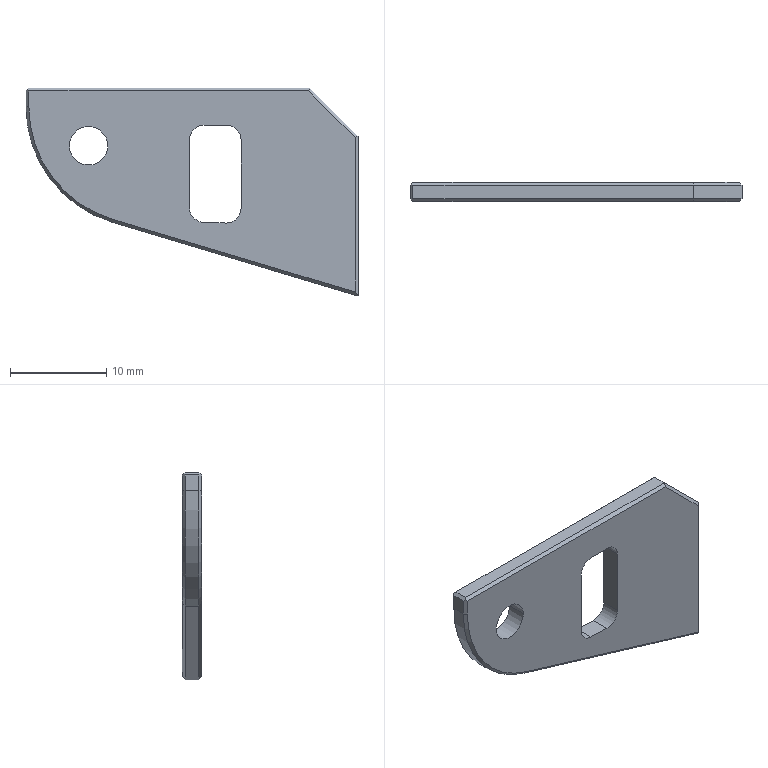Part | NX | 1 solid | 31 faces | box 34.5 x 2 x 21.6 mm | volume 937.237 mm3 | plane 22 | cylinder 7 | cone 2 | commonest cylinder face diameters 3 x4 4 x2 25 x1
STEP:
#1=CARTESIAN_POINT('',(-158.,156.8,-48.85));
#2=VERTEX_POINT('',#1);
#3=CARTESIAN_POINT('',(-158.,156.8,-47.2));
#4=VERTEX_POINT('',#3);
#5=CARTESIAN_POINT('',(-158.,156.8,-48.025));
#6=DIRECTION('',(0.,0.,1.));
#7=VECTOR('',#6,1000.);
#8=LINE('',#5,#7);
#9=EDGE_CURVE('',#2,#4,#8,.T.);
#10=ORIENTED_EDGE('',*,*,#9,.T.);
#11=CARTESIAN_POINT('',(-158.,158.2,-47.2));
#12=VERTEX_POINT('',#11);
#13=CARTESIAN_POINT('',(-158.,157.35,-47.2));
#14=DIRECTION('',(0.,1.,0.));
#15=VECTOR('',#14,1000.);
#16=LINE('',#13,#15);
#17=EDGE_CURVE('',#4,#12,#16,.T.);
#18=ORIENTED_EDGE('',*,*,#17,.T.);
#19=CARTESIAN_POINT('',(-158.,158.2,-48.85));
#20=VERTEX_POINT('',#19);
#21=CARTESIAN_POINT('',(-158.,158.2,-48.025));
#22=DIRECTION('',(0.,0.,1.));
#23=VECTOR('',#22,1000.);
#24=LINE('',#21,#23);
#25=EDGE_CURVE('',#20,#12,#24,.T.);
#26=ORIENTED_EDGE('',*,*,#25,.F.);
#27=CARTESIAN_POINT('',(-158.,156.5,-48.85));
#28=DIRECTION('',(0.,1.,0.));
#29=VECTOR('',#28,1000.);
#30=LINE('',#27,#29);
#31=EDGE_CURVE('',#2,#20,#30,.T.);
#32=ORIENTED_EDGE('',*,*,#31,.F.);
#33=EDGE_LOOP('',(#10,#18,#26,#32));
#34=FACE_BOUND('',#33,.T.);
#35=CARTESIAN_POINT('',(-158.,156.5,-42.9));
#36=DIRECTION('',(-1.,0.,0.));
#37=DIRECTION('',(0.,0.,1.));
#38=AXIS2_PLACEMENT_3D('',#35,#36,#37);
#39=PLANE('',#38);
#40=ADVANCED_FACE('',(#34),#39,.T.);
#41=CARTESIAN_POINT('',(-157.7,156.8,-46.9));
#42=VERTEX_POINT('',#41);
#43=CARTESIAN_POINT('',(-128.5,156.8,-46.9));
#44=VERTEX_POINT('',#43);
#45=CARTESIAN_POINT('',(-143.462,156.8,-46.9));
#46=DIRECTION('',(1.,0.,0.));
#47=VECTOR('',#46,1000.);
#48=LINE('',#45,#47);
#49=EDGE_CURVE('',#42,#44,#48,.T.);
#50=ORIENTED_EDGE('',*,*,#49,.T.);
#51=CARTESIAN_POINT('',(-128.5,158.2,-46.9));
#52=VERTEX_POINT('',#51);
#53=CARTESIAN_POINT('',(-128.5,157.5,-46.9));
#54=DIRECTION('',(0.,1.,0.));
#55=VECTOR('',#54,1000.);
#56=LINE('',#53,#55);
#57=EDGE_CURVE('',#44,#52,#56,.T.);
#58=ORIENTED_EDGE('',*,*,#57,.T.);
#59=CARTESIAN_POINT('',(-157.7,158.2,-46.9));
#60=VERTEX_POINT('',#59);
#61=CARTESIAN_POINT('',(-108.092,158.2,-46.9));
#62=DIRECTION('',(1.,0.,0.));
#63=VECTOR('',#62,1000.);
#64=LINE('',#61,#63);
#65=EDGE_CURVE('',#60,#52,#64,.T.);
#66=ORIENTED_EDGE('',*,*,#65,.F.);
#67=CARTESIAN_POINT('',(-157.7,157.35,-46.9));
#68=DIRECTION('',(0.,1.,0.));
#69=VECTOR('',#68,1000.);
#70=LINE('',#67,#69);
#71=EDGE_CURVE('',#42,#60,#70,.T.);
#72=ORIENTED_EDGE('',*,*,#71,.F.);
#73=EDGE_LOOP('',(#50,#58,#66,#72));
#74=FACE_BOUND('',#73,.T.);
#75=CARTESIAN_POINT('',(-123.5,156.5,-46.9));
#76=DIRECTION('',(0.,0.,1.));
#77=DIRECTION('',(0.,-1.,0.));
#78=AXIS2_PLACEMENT_3D('',#75,#76,#77);
#79=PLANE('',#78);
#80=ADVANCED_FACE('',(#74),#79,.T.);
#81=CARTESIAN_POINT('',(-123.5,158.2,-68.5));
#82=VERTEX_POINT('',#81);
#83=CARTESIAN_POINT('',(-123.5,156.8,-68.5));
#84=VERTEX_POINT('',#83);
#85=CARTESIAN_POINT('',(-123.5,156.5,-68.5));
#86=DIRECTION('',(0.,-1.,0.));
#87=VECTOR('',#86,1000.);
#88=LINE('',#85,#87);
#89=EDGE_CURVE('',#82,#84,#88,.T.);
#90=ORIENTED_EDGE('',*,*,#89,.F.);
#91=CARTESIAN_POINT('',(-123.5,158.2,-51.9));
#92=VERTEX_POINT('',#91);
#93=CARTESIAN_POINT('',(-123.5,158.2,-60.412));
#94=DIRECTION('',(0.,0.,-1.));
#95=VECTOR('',#94,1000.);
#96=LINE('',#93,#95);
#97=EDGE_CURVE('',#92,#82,#96,.T.);
#98=ORIENTED_EDGE('',*,*,#97,.F.);
#99=CARTESIAN_POINT('',(-123.5,156.8,-51.9));
#100=VERTEX_POINT('',#99);
#101=CARTESIAN_POINT('',(-123.5,157.5,-51.9));
#102=DIRECTION('',(0.,1.,0.));
#103=VECTOR('',#102,1000.);
#104=LINE('',#101,#103);
#105=EDGE_CURVE('',#100,#92,#104,.T.);
#106=ORIENTED_EDGE('',*,*,#105,.F.);
#107=CARTESIAN_POINT('',(-123.5,156.8,-60.412));
#108=DIRECTION('',(0.,0.,-1.));
#109=VECTOR('',#108,1000.);
#110=LINE('',#107,#109);
#111=EDGE_CURVE('',#100,#84,#110,.T.);
#112=ORIENTED_EDGE('',*,*,#111,.T.);
#113=EDGE_LOOP('',(#90,#98,#106,#112));
#114=FACE_BOUND('',#113,.T.);
#115=CARTESIAN_POINT('',(-123.5,156.5,-67.9));
#116=DIRECTION('',(1.,0.,0.));
#117=DIRECTION('',(0.,1.,0.));
#118=AXIS2_PLACEMENT_3D('',#115,#116,#117);
#119=PLANE('',#118);
#120=ADVANCED_FACE('',(#114),#119,.T.);
#121=CARTESIAN_POINT('',(-135.65,156.5,-59.427));
#122=VERTEX_POINT('',#121);
#123=CARTESIAN_POINT('',(-135.65,158.5,-59.427));
#124=VERTEX_POINT('',#123);
#125=CARTESIAN_POINT('',(-135.65,156.5,-59.427));
#126=DIRECTION('',(0.,1.,0.));
#127=VECTOR('',#126,1000.);
#128=LINE('',#125,#127);
#129=EDGE_CURVE('',#122,#124,#128,.T.);
#130=ORIENTED_EDGE('',*,*,#129,.T.);
#131=CARTESIAN_POINT('',(-137.197,158.5,-60.926));
#132=VERTEX_POINT('',#131);
#133=CARTESIAN_POINT('',(-137.15,158.5,-59.427));
#134=DIRECTION('',(0.,1.,0.));
#135=DIRECTION('',(-1.,0.,0.));
#136=AXIS2_PLACEMENT_3D('',#133,#134,#135);
#137=CIRCLE('',#136,1.5);
#138=EDGE_CURVE('',#124,#132,#137,.T.);
#139=ORIENTED_EDGE('',*,*,#138,.T.);
#140=CARTESIAN_POINT('',(-137.197,156.5,-60.926));
#141=VERTEX_POINT('',#140);
#142=CARTESIAN_POINT('',(-137.197,156.5,-60.926));
#143=DIRECTION('',(0.,1.,0.));
#144=VECTOR('',#143,1000.);
#145=LINE('',#142,#144);
#146=EDGE_CURVE('',#141,#132,#145,.T.);
#147=ORIENTED_EDGE('',*,*,#146,.F.);
#148=CARTESIAN_POINT('',(-137.15,156.5,-59.427));
#149=DIRECTION('',(0.,1.,0.));
#150=DIRECTION('',(-1.,0.,0.));
#151=AXIS2_PLACEMENT_3D('',#148,#149,#150);
#152=CIRCLE('',#151,1.5);
#153=EDGE_CURVE('',#122,#141,#152,.T.);
#154=ORIENTED_EDGE('',*,*,#153,.F.);
#155=EDGE_LOOP('',(#130,#139,#147,#154));
#156=FACE_BOUND('',#155,.T.);
#157=CARTESIAN_POINT('',(-137.15,156.5,-59.427));
#158=DIRECTION('',(0.,1.,0.));
#159=DIRECTION('',(-1.,0.,0.));
#160=AXIS2_PLACEMENT_3D('',#157,#158,#159);
#161=CYLINDRICAL_SURFACE('',#160,1.5);
#162=ADVANCED_FACE('',(#156),#161,.F.);
#163=CARTESIAN_POINT('',(-149.092,156.8,-60.822));
#164=VERTEX_POINT('',#163);
#165=CARTESIAN_POINT('',(-136.446,156.8,-64.616));
#166=DIRECTION('',(-0.9578,0.,0.2873));
#167=VECTOR('',#166,1000.);
#168=LINE('',#165,#167);
#169=EDGE_CURVE('',#84,#164,#168,.T.);
#170=ORIENTED_EDGE('',*,*,#169,.T.);
#171=CARTESIAN_POINT('',(-149.092,158.2,-60.822));
#172=VERTEX_POINT('',#171);
#173=CARTESIAN_POINT('',(-149.092,156.5,-60.822));
#174=DIRECTION('',(0.,1.,0.));
#175=VECTOR('',#174,1000.);
#176=LINE('',#173,#175);
#177=EDGE_CURVE('',#164,#172,#176,.T.);
#178=ORIENTED_EDGE('',*,*,#177,.T.);
#179=CARTESIAN_POINT('',(-136.446,158.2,-64.616));
#180=DIRECTION('',(0.9578,0.,-0.2873));
#181=VECTOR('',#180,1000.);
#182=LINE('',#179,#181);
#183=EDGE_CURVE('',#172,#82,#182,.T.);
#184=ORIENTED_EDGE('',*,*,#183,.T.);
#185=ORIENTED_EDGE('',*,*,#89,.T.);
#186=EDGE_LOOP('',(#170,#178,#184,#185));
#187=FACE_BOUND('',#186,.T.);
#188=CARTESIAN_POINT('',(-160.5,156.5,-57.4));
#189=DIRECTION('',(-0.2873,0.,-0.9578));
#190=DIRECTION('',(-0.9578,0.,0.2873));
#191=AXIS2_PLACEMENT_3D('',#188,#189,#190);
#192=PLANE('',#191);
#193=ADVANCED_FACE('',(#187),#192,.T.);
#194=CARTESIAN_POINT('',(-141.001,156.5,-59.354));
#195=VERTEX_POINT('',#194);
#196=CARTESIAN_POINT('',(-141.001,158.5,-59.354));
#197=VERTEX_POINT('',#196);
#198=CARTESIAN_POINT('',(-141.001,156.5,-59.354));
#199=DIRECTION('',(0.,1.,0.));
#200=VECTOR('',#199,1000.);
#201=LINE('',#198,#200);
#202=EDGE_CURVE('',#195,#197,#201,.T.);
#203=ORIENTED_EDGE('',*,*,#202,.F.);
#204=CARTESIAN_POINT('',(-139.548,156.5,-60.853));
#205=VERTEX_POINT('',#204);
#206=CARTESIAN_POINT('',(-139.501,156.5,-59.354));
#207=DIRECTION('',(0.,1.,0.));
#208=DIRECTION('',(-1.,0.,0.));
#209=AXIS2_PLACEMENT_3D('',#206,#207,#208);
#210=CIRCLE('',#209,1.5);
#211=EDGE_CURVE('',#205,#195,#210,.T.);
#212=ORIENTED_EDGE('',*,*,#211,.F.);
#213=CARTESIAN_POINT('',(-139.548,158.5,-60.853));
#214=VERTEX_POINT('',#213);
#215=CARTESIAN_POINT('',(-139.548,156.5,-60.853));
#216=DIRECTION('',(0.,1.,0.));
#217=VECTOR('',#216,1000.);
#218=LINE('',#215,#217);
#219=EDGE_CURVE('',#205,#214,#218,.T.);
#220=ORIENTED_EDGE('',*,*,#219,.T.);
#221=CARTESIAN_POINT('',(-139.501,158.5,-59.354));
#222=DIRECTION('',(0.,1.,0.));
#223=DIRECTION('',(-1.,0.,0.));
#224=AXIS2_PLACEMENT_3D('',#221,#222,#223);
#225=CIRCLE('',#224,1.5);
#226=EDGE_CURVE('',#214,#197,#225,.T.);
#227=ORIENTED_EDGE('',*,*,#226,.T.);
#228=EDGE_LOOP('',(#203,#212,#220,#227));
#229=FACE_BOUND('',#228,.T.);
#230=CARTESIAN_POINT('',(-139.501,156.5,-59.354));
#231=DIRECTION('',(0.,1.,0.));
#232=DIRECTION('',(-1.,0.,0.));
#233=AXIS2_PLACEMENT_3D('',#230,#231,#232);
#234=CYLINDRICAL_SURFACE('',#233,1.5);
#235=ADVANCED_FACE('',(#229),#234,.F.);
#236=CARTESIAN_POINT('',(-137.15,156.5,-50.763));
#237=VERTEX_POINT('',#236);
#238=CARTESIAN_POINT('',(-137.15,158.5,-50.763));
#239=VERTEX_POINT('',#238);
#240=CARTESIAN_POINT('',(-137.15,156.5,-50.763));
#241=DIRECTION('',(0.,1.,0.));
#242=VECTOR('',#241,1000.);
#243=LINE('',#240,#242);
#244=EDGE_CURVE('',#237,#239,#243,.T.);
#245=ORIENTED_EDGE('',*,*,#244,.F.);
#246=CARTESIAN_POINT('',(-139.501,156.5,-50.763));
#247=VERTEX_POINT('',#246);
#248=CARTESIAN_POINT('',(-108.092,156.5,-50.763));
#249=DIRECTION('',(1.,0.,0.));
#250=VECTOR('',#249,1000.);
#251=LINE('',#248,#250);
#252=EDGE_CURVE('',#247,#237,#251,.T.);
#253=ORIENTED_EDGE('',*,*,#252,.F.);
#254=CARTESIAN_POINT('',(-139.501,158.5,-50.763));
#255=VERTEX_POINT('',#254);
#256=CARTESIAN_POINT('',(-139.501,156.5,-50.763));
#257=DIRECTION('',(0.,1.,0.));
#258=VECTOR('',#257,1000.);
#259=LINE('',#256,#258);
#260=EDGE_CURVE('',#247,#255,#259,.T.);
#261=ORIENTED_EDGE('',*,*,#260,.T.);
#262=CARTESIAN_POINT('',(-108.092,158.5,-50.763));
#263=DIRECTION('',(1.,0.,0.));
#264=VECTOR('',#263,1000.);
#265=LINE('',#262,#264);
#266=EDGE_CURVE('',#255,#239,#265,.T.);
#267=ORIENTED_EDGE('',*,*,#266,.T.);
#268=EDGE_LOOP('',(#245,#253,#261,#267));
#269=FACE_BOUND('',#268,.T.);
#270=CARTESIAN_POINT('',(-135.65,156.3,-50.763));
#271=DIRECTION('',(0.,0.,1.));
#272=DIRECTION('',(0.,-1.,0.));
#273=AXIS2_PLACEMENT_3D('',#270,#271,#272);
#274=PLANE('',#273);
#275=ADVANCED_FACE('',(#269),#274,.F.);
#276=ORIENTED_EDGE('',*,*,#129,.F.);
#277=CARTESIAN_POINT('',(-135.65,156.5,-52.263));
#278=VERTEX_POINT('',#277);
#279=CARTESIAN_POINT('',(-135.65,156.5,-58.685));
#280=DIRECTION('',(0.,0.,-1.));
#281=VECTOR('',#280,1000.);
#282=LINE('',#279,#281);
#283=EDGE_CURVE('',#278,#122,#282,.T.);
#284=ORIENTED_EDGE('',*,*,#283,.F.);
#285=CARTESIAN_POINT('',(-135.65,158.5,-52.263));
#286=VERTEX_POINT('',#285);
#287=CARTESIAN_POINT('',(-135.65,156.5,-52.263));
#288=DIRECTION('',(0.,1.,0.));
#289=VECTOR('',#288,1000.);
#290=LINE('',#287,#289);
#291=EDGE_CURVE('',#278,#286,#290,.T.);
#292=ORIENTED_EDGE('',*,*,#291,.T.);
#293=CARTESIAN_POINT('',(-135.65,158.5,-58.685));
#294=DIRECTION('',(0.,0.,-1.));
#295=VECTOR('',#294,1000.);
#296=LINE('',#293,#295);
#297=EDGE_CURVE('',#286,#124,#296,.T.);
#298=ORIENTED_EDGE('',*,*,#297,.T.);
#299=EDGE_LOOP('',(#276,#284,#292,#298));
#300=FACE_BOUND('',#299,.T.);
#301=CARTESIAN_POINT('',(-135.65,156.3,-60.975));
#302=DIRECTION('',(1.,0.,0.));
#303=DIRECTION('',(0.,0.,-1.));
#304=AXIS2_PLACEMENT_3D('',#301,#302,#303);
#305=PLANE('',#304);
#306=ADVANCED_FACE('',(#300),#305,.F.);
#307=CARTESIAN_POINT('',(-108.092,158.5,-61.836));
#308=DIRECTION('',(-0.9995,0.,0.03124));
#309=VECTOR('',#308,1000.);
#310=LINE('',#307,#309);
#311=EDGE_CURVE('',#132,#214,#310,.T.);
#312=ORIENTED_EDGE('',*,*,#311,.T.);
#313=ORIENTED_EDGE('',*,*,#219,.F.);
#314=CARTESIAN_POINT('',(-108.092,156.5,-61.836));
#315=DIRECTION('',(-0.9995,0.,0.03124));
#316=VECTOR('',#315,1000.);
#317=LINE('',#314,#316);
#318=EDGE_CURVE('',#141,#205,#317,.T.);
#319=ORIENTED_EDGE('',*,*,#318,.F.);
#320=ORIENTED_EDGE('',*,*,#146,.T.);
#321=EDGE_LOOP('',(#312,#313,#319,#320));
#322=FACE_BOUND('',#321,.T.);
#323=CARTESIAN_POINT('',(-141.001,156.3,-60.807));
#324=DIRECTION('',(-0.03124,0.,-0.9995));
#325=DIRECTION('',(-0.9995,0.,0.03124));
#326=AXIS2_PLACEMENT_3D('',#323,#324,#325);
#327=PLANE('',#326);
#328=ADVANCED_FACE('',(#322),#327,.F.);
#329=ORIENTED_EDGE('',*,*,#202,.T.);
#330=CARTESIAN_POINT('',(-141.001,158.5,-52.263));
#331=VERTEX_POINT('',#330);
#332=CARTESIAN_POINT('',(-141.001,158.5,-58.685));
#333=DIRECTION('',(0.,0.,1.));
#334=VECTOR('',#333,1000.);
#335=LINE('',#332,#334);
#336=EDGE_CURVE('',#197,#331,#335,.T.);
#337=ORIENTED_EDGE('',*,*,#336,.T.);
#338=CARTESIAN_POINT('',(-141.001,156.5,-52.263));
#339=VERTEX_POINT('',#338);
#340=CARTESIAN_POINT('',(-141.001,156.5,-52.263));
#341=DIRECTION('',(0.,1.,0.));
#342=VECTOR('',#341,1000.);
#343=LINE('',#340,#342);
#344=EDGE_CURVE('',#339,#331,#343,.T.);
#345=ORIENTED_EDGE('',*,*,#344,.F.);
#346=CARTESIAN_POINT('',(-141.001,156.5,-58.685));
#347=DIRECTION('',(0.,0.,1.));
#348=VECTOR('',#347,1000.);
#349=LINE('',#346,#348);
#350=EDGE_CURVE('',#195,#339,#349,.T.);
#351=ORIENTED_EDGE('',*,*,#350,.F.);
#352=EDGE_LOOP('',(#329,#337,#345,#351));
#353=FACE_BOUND('',#352,.T.);
#354=CARTESIAN_POINT('',(-141.001,156.3,-50.763));
#355=DIRECTION('',(-1.,0.,0.));
#356=DIRECTION('',(0.,0.,1.));
#357=AXIS2_PLACEMENT_3D('',#354,#355,#356);
#358=PLANE('',#357);
#359=ADVANCED_FACE('',(#353),#358,.F.);
#360=ORIENTED_EDGE('',*,*,#344,.T.);
#361=CARTESIAN_POINT('',(-139.501,158.5,-52.263));
#362=DIRECTION('',(0.,1.,0.));
#363=DIRECTION('',(-1.,0.,0.));
#364=AXIS2_PLACEMENT_3D('',#361,#362,#363);
#365=CIRCLE('',#364,1.5);
#366=EDGE_CURVE('',#331,#255,#365,.T.);
#367=ORIENTED_EDGE('',*,*,#366,.T.);
#368=ORIENTED_EDGE('',*,*,#260,.F.);
#369=CARTESIAN_POINT('',(-139.501,156.5,-52.263));
#370=DIRECTION('',(0.,1.,0.));
#371=DIRECTION('',(-1.,0.,0.));
#372=AXIS2_PLACEMENT_3D('',#369,#370,#371);
#373=CIRCLE('',#372,1.5);
#374=EDGE_CURVE('',#339,#247,#373,.T.);
#375=ORIENTED_EDGE('',*,*,#374,.F.);
#376=EDGE_LOOP('',(#360,#367,#368,#375));
#377=FACE_BOUND('',#376,.T.);
#378=CARTESIAN_POINT('',(-139.501,156.5,-52.263));
#379=DIRECTION('',(0.,1.,0.));
#380=DIRECTION('',(-1.,0.,0.));
#381=AXIS2_PLACEMENT_3D('',#378,#379,#380);
#382=CYLINDRICAL_SURFACE('',#381,1.5);
#383=ADVANCED_FACE('',(#377),#382,.F.);
#384=ORIENTED_EDGE('',*,*,#244,.T.);
#385=CARTESIAN_POINT('',(-137.15,158.5,-52.263));
#386=DIRECTION('',(0.,1.,0.));
#387=DIRECTION('',(-1.,0.,0.));
#388=AXIS2_PLACEMENT_3D('',#385,#386,#387);
#389=CIRCLE('',#388,1.5);
#390=EDGE_CURVE('',#239,#286,#389,.T.);
#391=ORIENTED_EDGE('',*,*,#390,.T.);
#392=ORIENTED_EDGE('',*,*,#291,.F.);
#393=CARTESIAN_POINT('',(-137.15,156.5,-52.263));
#394=DIRECTION('',(0.,1.,0.));
#395=DIRECTION('',(-1.,0.,0.));
#396=AXIS2_PLACEMENT_3D('',#393,#394,#395);
#397=CIRCLE('',#396,1.5);
#398=EDGE_CURVE('',#237,#278,#397,.T.);
#399=ORIENTED_EDGE('',*,*,#398,.F.);
#400=EDGE_LOOP('',(#384,#391,#392,#399));
#401=FACE_BOUND('',#400,.T.);
#402=CARTESIAN_POINT('',(-137.15,156.5,-52.263));
#403=DIRECTION('',(0.,1.,0.));
#404=DIRECTION('',(-1.,0.,0.));
#405=AXIS2_PLACEMENT_3D('',#402,#403,#404);
#406=CYLINDRICAL_SURFACE('',#405,1.5);
#407=ADVANCED_FACE('',(#401),#406,.F.);
#408=CARTESIAN_POINT('',(-126.,158.2,-49.4));
#409=DIRECTION('',(-0.7071,0.,0.7071));
#410=VECTOR('',#409,1000.);
#411=LINE('',#408,#410);
#412=EDGE_CURVE('',#92,#52,#411,.T.);
#413=ORIENTED_EDGE('',*,*,#412,.T.);
#414=ORIENTED_EDGE('',*,*,#57,.F.);
#415=CARTESIAN_POINT('',(-126.,156.8,-49.4));
#416=DIRECTION('',(-0.7071,0.,0.7071));
#417=VECTOR('',#416,1000.);
#418=LINE('',#415,#417);
#419=EDGE_CURVE('',#100,#44,#418,.T.);
#420=ORIENTED_EDGE('',*,*,#419,.F.);
#421=ORIENTED_EDGE('',*,*,#105,.T.);
#422=EDGE_LOOP('',(#413,#414,#420,#421));
#423=FACE_BOUND('',#422,.T.);
#424=CARTESIAN_POINT('',(-126.,157.5,-49.4));
#425=DIRECTION('',(0.7071,0.,0.7071));
#426=DIRECTION('',(0.,-1.,0.));
#427=AXIS2_PLACEMENT_3D('',#424,#425,#426);
#428=PLANE('',#427);
#429=ADVANCED_FACE('',(#423),#428,.T.);
#430=CARTESIAN_POINT('',(-128.624,158.5,-47.2));
#431=VERTEX_POINT('',#430);
#432=CARTESIAN_POINT('',(-133.381,169.985,-58.685));
#433=DIRECTION('',(-0.2811,0.6786,-0.6786));
#434=VECTOR('',#433,1000.);
#435=LINE('',#432,#434);
#436=EDGE_CURVE('',#52,#431,#435,.T.);
#437=ORIENTED_EDGE('',*,*,#436,.F.);
#438=ORIENTED_EDGE('',*,*,#412,.F.);
#439=CARTESIAN_POINT('',(-123.8,158.5,-52.024));
#440=VERTEX_POINT('',#439);
#441=CARTESIAN_POINT('',(-108.092,142.792,-45.518));
#442=DIRECTION('',(0.6786,-0.6786,0.2811));
#443=VECTOR('',#442,1000.);
#444=LINE('',#441,#443);
#445=EDGE_CURVE('',#440,#92,#444,.T.);
#446=ORIENTED_EDGE('',*,*,#445,.F.);
#447=CARTESIAN_POINT('',(-117.139,158.5,-58.685));
#448=DIRECTION('',(-0.7071,0.,0.7071));
#449=VECTOR('',#448,1000.);
#450=LINE('',#447,#449);
#451=EDGE_CURVE('',#440,#431,#450,.T.);
#452=ORIENTED_EDGE('',*,*,#451,.T.);
#453=EDGE_LOOP('',(#437,#438,#446,#452));
#454=FACE_BOUND('',#453,.T.);
#455=CARTESIAN_POINT('',(-126.106,158.35,-49.506));
#456=DIRECTION('',(0.5,0.7071,0.5));
#457=DIRECTION('',(0.7071,0.,-0.7071));
#458=AXIS2_PLACEMENT_3D('',#455,#456,#457);
#459=PLANE('',#458);
#460=ADVANCED_FACE('',(#454),#459,.T.);
#461=ORIENTED_EDGE('',*,*,#419,.T.);
#462=CARTESIAN_POINT('',(-128.624,156.5,-47.2));
#463=VERTEX_POINT('',#462);
#464=CARTESIAN_POINT('',(-133.381,145.015,-58.685));
#465=DIRECTION('',(0.2811,0.6786,0.6786));
#466=VECTOR('',#465,1000.);
#467=LINE('',#464,#466);
#468=EDGE_CURVE('',#463,#44,#467,.T.);
#469=ORIENTED_EDGE('',*,*,#468,.F.);
#470=CARTESIAN_POINT('',(-123.8,156.5,-52.024));
#471=VERTEX_POINT('',#470);
#472=CARTESIAN_POINT('',(-117.139,156.5,-58.685));
#473=DIRECTION('',(-0.7071,0.,0.7071));
#474=VECTOR('',#473,1000.);
#475=LINE('',#472,#474);
#476=EDGE_CURVE('',#471,#463,#475,.T.);
#477=ORIENTED_EDGE('',*,*,#476,.F.);
#478=CARTESIAN_POINT('',(-108.092,172.208,-45.518));
#479=DIRECTION('',(-0.6786,-0.6786,-0.2811));
#480=VECTOR('',#479,1000.);
#481=LINE('',#478,#480);
#482=EDGE_CURVE('',#100,#471,#481,.T.);
#483=ORIENTED_EDGE('',*,*,#482,.F.);
#484=EDGE_LOOP('',(#461,#469,#477,#483));
#485=FACE_BOUND('',#484,.T.);
#486=CARTESIAN_POINT('',(-126.106,156.65,-49.506));
#487=DIRECTION('',(-0.5,0.7071,-0.5));
#488=DIRECTION('',(-0.7071,0.,0.7071));
#489=AXIS2_PLACEMENT_3D('',#486,#487,#488);
#490=PLANE('',#489);
#491=ADVANCED_FACE('',(#485),#490,.F.);
#492=ORIENTED_EDGE('',*,*,#17,.F.);
#493=CARTESIAN_POINT('',(-157.85,156.65,-47.05));
#494=VERTEX_POINT('',#493);
#495=CARTESIAN_POINT('',(-169.485,168.285,-58.685));
#496=DIRECTION('',(-0.5774,0.5774,-0.5774));
#497=VECTOR('',#496,1000.);
#498=LINE('',#495,#497);
#499=EDGE_CURVE('',#494,#4,#498,.T.);
#500=ORIENTED_EDGE('',*,*,#499,.F.);
#501=CARTESIAN_POINT('',(-169.485,145.015,-58.685));
#502=DIRECTION('',(-0.5774,-0.5774,-0.5774));
#503=VECTOR('',#502,1000.);
#504=LINE('',#501,#503);
#505=EDGE_CURVE('',#42,#494,#504,.T.);
#506=ORIENTED_EDGE('',*,*,#505,.F.);
#507=ORIENTED_EDGE('',*,*,#71,.T.);
#508=CARTESIAN_POINT('',(-157.85,158.35,-47.05));
#509=VERTEX_POINT('',#508);
#510=CARTESIAN_POINT('',(-169.485,169.985,-58.685));
#511=DIRECTION('',(-0.5774,0.5774,-0.5774));
#512=VECTOR('',#511,1000.);
#513=LINE('',#510,#512);
#514=EDGE_CURVE('',#60,#509,#513,.T.);
#515=ORIENTED_EDGE('',*,*,#514,.T.);
#516=CARTESIAN_POINT('',(-169.485,146.715,-58.685));
#517=DIRECTION('',(0.5774,0.5774,0.5774));
#518=VECTOR('',#517,1000.);
#519=LINE('',#516,#518);
#520=EDGE_CURVE('',#12,#509,#519,.T.);
#521=ORIENTED_EDGE('',*,*,#520,.F.);
#522=EDGE_LOOP('',(#492,#500,#506,#507,#515,#521));
#523=FACE_BOUND('',#522,.T.);
#524=CARTESIAN_POINT('',(-157.85,157.35,-47.05));
#525=DIRECTION('',(-0.7071,0.,0.7071));
#526=DIRECTION('',(0.,1.,0.));
#527=AXIS2_PLACEMENT_3D('',#524,#525,#526);
#528=PLANE('',#527);
#529=ADVANCED_FACE('',(#523),#528,.T.);
#530=CARTESIAN_POINT('',(-145.5,156.8,-48.85));
#531=DIRECTION('',(0.,1.,0.));
#532=DIRECTION('',(-1.,0.,0.));
#533=AXIS2_PLACEMENT_3D('',#530,#531,#532);
#534=CIRCLE('',#533,12.5);
#535=EDGE_CURVE('',#164,#2,#534,.T.);
#536=ORIENTED_EDGE('',*,*,#535,.T.);
#537=ORIENTED_EDGE('',*,*,#31,.T.);
#538=CARTESIAN_POINT('',(-145.5,158.2,-48.85));
#539=DIRECTION('',(0.,1.,0.));
#540=DIRECTION('',(-1.,0.,0.));
#541=AXIS2_PLACEMENT_3D('',#538,#539,#540);
#542=CIRCLE('',#541,12.5);
#543=EDGE_CURVE('',#172,#20,#542,.T.);
#544=ORIENTED_EDGE('',*,*,#543,.F.);
#545=ORIENTED_EDGE('',*,*,#177,.F.);
#546=EDGE_LOOP('',(#536,#537,#544,#545));
#547=FACE_BOUND('',#546,.T.);
#548=CARTESIAN_POINT('',(-145.5,156.5,-48.85));
#549=DIRECTION('',(0.,1.,0.));
#550=DIRECTION('',(-1.,0.,0.));
#551=AXIS2_PLACEMENT_3D('',#548,#549,#550);
#552=CYLINDRICAL_SURFACE('',#551,12.5);
#553=ADVANCED_FACE('',(#547),#552,.T.);
#554=ORIENTED_EDGE('',*,*,#183,.F.);
#555=CARTESIAN_POINT('',(-149.006,158.5,-60.535));
#556=VERTEX_POINT('',#555);
#557=CARTESIAN_POINT('',(-149.092,158.2,-60.822));
#558=DIRECTION('',(0.2032,0.7071,0.6773));
#559=VECTOR('',#558,1000.);
#560=LINE('',#557,#559);
#561=EDGE_CURVE('',#172,#556,#560,.T.);
#562=ORIENTED_EDGE('',*,*,#561,.T.);
#563=CARTESIAN_POINT('',(-123.8,158.5,-68.097));
#564=VERTEX_POINT('',#563);
#565=CARTESIAN_POINT('',(-136.36,158.5,-64.329));
#566=DIRECTION('',(0.9578,0.,-0.2873));
#567=VECTOR('',#566,1000.);
#568=LINE('',#565,#567);
#569=EDGE_CURVE('',#556,#564,#568,.T.);
#570=ORIENTED_EDGE('',*,*,#569,.T.);
#571=CARTESIAN_POINT('',(-130.803,165.503,-58.685));
#572=DIRECTION('',(0.5126,-0.5126,-0.6889));
#573=VECTOR('',#572,1000.);
#574=LINE('',#571,#573);
#575=EDGE_CURVE('',#564,#82,#574,.T.);
#576=ORIENTED_EDGE('',*,*,#575,.T.);
#577=EDGE_LOOP('',(#554,#562,#570,#576));
#578=FACE_BOUND('',#577,.T.);
#579=CARTESIAN_POINT('',(-136.403,158.35,-64.473));
#580=DIRECTION('',(-0.2032,0.7071,-0.6773));
#581=DIRECTION('',(-0.9578,0.,0.2873));
#582=AXIS2_PLACEMENT_3D('',#579,#580,#581);
#583=PLANE('',#582);
#584=ADVANCED_FACE('',(#578),#583,.T.);
#585=ORIENTED_EDGE('',*,*,#543,.T.);
#586=CARTESIAN_POINT('',(-157.7,158.5,-48.85));
#587=VERTEX_POINT('',#586);
#588=CARTESIAN_POINT('',(-157.7,158.5,-48.85));
#589=DIRECTION('',(-0.7071,-0.7071,0.));
#590=VECTOR('',#589,1000.);
#591=LINE('',#588,#590);
#592=EDGE_CURVE('',#587,#20,#591,.T.);
#593=ORIENTED_EDGE('',*,*,#592,.F.);
#594=CARTESIAN_POINT('',(-145.5,158.5,-48.85));
#595=DIRECTION('',(0.,1.,0.));
#596=DIRECTION('',(-1.,0.,0.));
#597=AXIS2_PLACEMENT_3D('',#594,#595,#596);
#598=CIRCLE('',#597,12.2);
#599=EDGE_CURVE('',#556,#587,#598,.T.);
#600=ORIENTED_EDGE('',*,*,#599,.F.);
#601=ORIENTED_EDGE('',*,*,#561,.F.);
#602=EDGE_LOOP('',(#585,#593,#600,#601));
#603=FACE_BOUND('',#602,.T.);
#604=CARTESIAN_POINT('',(-145.5,158.2,-48.85));
#605=DIRECTION('',(0.,-1.,0.));
#606=DIRECTION('',(1.,0.,0.));
#607=AXIS2_PLACEMENT_3D('',#604,#605,#606);
#608=CONICAL_SURFACE('',#607,12.5,0.7854);
#609=ADVANCED_FACE('',(#603),#608,.T.);
#610=ORIENTED_EDGE('',*,*,#169,.F.);
#611=CARTESIAN_POINT('',(-123.8,156.5,-68.097));
#612=VERTEX_POINT('',#611);
#613=CARTESIAN_POINT('',(-130.803,149.497,-58.685));
#614=DIRECTION('',(0.5126,0.5126,-0.6889));
#615=VECTOR('',#614,1000.);
#616=LINE('',#613,#615);
#617=EDGE_CURVE('',#612,#84,#616,.T.);
#618=ORIENTED_EDGE('',*,*,#617,.F.);
#619=CARTESIAN_POINT('',(-149.006,156.5,-60.535));
#620=VERTEX_POINT('',#619);
#621=CARTESIAN_POINT('',(-136.36,156.5,-64.329));
#622=DIRECTION('',(-0.9578,0.,0.2873));
#623=VECTOR('',#622,1000.);
#624=LINE('',#621,#623);
#625=EDGE_CURVE('',#612,#620,#624,.T.);
#626=ORIENTED_EDGE('',*,*,#625,.T.);
#627=CARTESIAN_POINT('',(-149.006,156.5,-60.535));
#628=DIRECTION('',(-0.2032,0.7071,-0.6773));
#629=VECTOR('',#628,1000.);
#630=LINE('',#627,#629);
#631=EDGE_CURVE('',#620,#164,#630,.T.);
#632=ORIENTED_EDGE('',*,*,#631,.T.);
#633=EDGE_LOOP('',(#610,#618,#626,#632));
#634=FACE_BOUND('',#633,.T.);
#635=CARTESIAN_POINT('',(-136.403,156.65,-64.473));
#636=DIRECTION('',(-0.2032,-0.7071,-0.6773));
#637=DIRECTION('',(0.,0.6917,-0.7222));
#638=AXIS2_PLACEMENT_3D('',#635,#636,#637);
#639=PLANE('',#638);
#640=ADVANCED_FACE('',(#634),#639,.T.);
#641=ORIENTED_EDGE('',*,*,#535,.F.);
#642=ORIENTED_EDGE('',*,*,#631,.F.);
#643=CARTESIAN_POINT('',(-157.7,156.5,-48.85));
#644=VERTEX_POINT('',#643);
#645=CARTESIAN_POINT('',(-145.5,156.5,-48.85));
#646=DIRECTION('',(0.,1.,0.));
#647=DIRECTION('',(-1.,0.,0.));
#648=AXIS2_PLACEMENT_3D('',#645,#646,#647);
#649=CIRCLE('',#648,12.2);
#650=EDGE_CURVE('',#620,#644,#649,.T.);
#651=ORIENTED_EDGE('',*,*,#650,.T.);
#652=CARTESIAN_POINT('',(-157.7,156.5,-48.85));
#653=DIRECTION('',(-0.7071,0.7071,0.));
#654=VECTOR('',#653,1000.);
#655=LINE('',#652,#654);
#656=EDGE_CURVE('',#644,#2,#655,.T.);
#657=ORIENTED_EDGE('',*,*,#656,.T.);
#658=EDGE_LOOP('',(#641,#642,#651,#657));
#659=FACE_BOUND('',#658,.T.);
#660=CARTESIAN_POINT('',(-145.5,156.8,-48.85));
#661=DIRECTION('',(0.,1.,0.));
#662=DIRECTION('',(-1.,0.,0.));
#663=AXIS2_PLACEMENT_3D('',#660,#661,#662);
#664=CONICAL_SURFACE('',#663,12.5,0.7854);
#665=ADVANCED_FACE('',(#659),#664,.T.);
#666=ORIENTED_EDGE('',*,*,#9,.F.);
#667=ORIENTED_EDGE('',*,*,#656,.F.);
#668=CARTESIAN_POINT('',(-157.7,156.5,-47.2));
#669=VERTEX_POINT('',#668);
#670=CARTESIAN_POINT('',(-157.7,156.5,-48.025));
#671=DIRECTION('',(0.,0.,1.));
#672=VECTOR('',#671,1000.);
#673=LINE('',#670,#672);
#674=EDGE_CURVE('',#644,#669,#673,.T.);
#675=ORIENTED_EDGE('',*,*,#674,.T.);
#676=CARTESIAN_POINT('',(-146.215,145.015,-58.685));
#677=DIRECTION('',(0.5774,-0.5774,-0.5774));
#678=VECTOR('',#677,1000.);
#679=LINE('',#676,#678);
#680=EDGE_CURVE('',#494,#669,#679,.T.);
#681=ORIENTED_EDGE('',*,*,#680,.F.);
#682=ORIENTED_EDGE('',*,*,#499,.T.);
#683=EDGE_LOOP('',(#666,#667,#675,#681,#682));
#684=FACE_BOUND('',#683,.T.);
#685=CARTESIAN_POINT('',(-157.85,156.65,-48.025));
#686=DIRECTION('',(-0.7071,-0.7071,0.));
#687=DIRECTION('',(-0.7071,0.7071,0.));
#688=AXIS2_PLACEMENT_3D('',#685,#686,#687);
#689=PLANE('',#688);
#690=ADVANCED_FACE('',(#684),#689,.T.);
#691=CARTESIAN_POINT('',(-149.5,158.5,-52.9));
#692=VERTEX_POINT('',#691);
#693=CARTESIAN_POINT('',(-153.5,158.5,-52.9));
#694=VERTEX_POINT('',#693);
#695=CARTESIAN_POINT('',(-151.5,158.5,-52.9));
#696=DIRECTION('',(0.,1.,0.));
#697=DIRECTION('',(-1.,0.,0.));
#698=AXIS2_PLACEMENT_3D('',#695,#696,#697);
#699=CIRCLE('',#698,2.);
#700=EDGE_CURVE('',#692,#694,#699,.T.);
#701=ORIENTED_EDGE('',*,*,#700,.T.);
#702=CARTESIAN_POINT('',(-153.5,156.5,-52.9));
#703=VERTEX_POINT('',#702);
#704=CARTESIAN_POINT('',(-153.5,156.5,-52.9));
#705=DIRECTION('',(0.,1.,0.));
#706=VECTOR('',#705,1000.);
#707=LINE('',#704,#706);
#708=EDGE_CURVE('',#694,#703,#707,.F.);
#709=ORIENTED_EDGE('',*,*,#708,.T.);
#710=CARTESIAN_POINT('',(-149.5,156.5,-52.9));
#711=VERTEX_POINT('',#710);
#712=CARTESIAN_POINT('',(-151.5,156.5,-52.9));
#713=DIRECTION('',(0.,1.,0.));
#714=DIRECTION('',(-1.,0.,0.));
#715=AXIS2_PLACEMENT_3D('',#712,#713,#714);
#716=CIRCLE('',#715,2.);
#717=EDGE_CURVE('',#711,#703,#716,.T.);
#718=ORIENTED_EDGE('',*,*,#717,.F.);
#719=CARTESIAN_POINT('',(-149.5,156.5,-52.9));
#720=DIRECTION('',(0.,1.,0.));
#721=VECTOR('',#720,1000.);
#722=LINE('',#719,#721);
#723=EDGE_CURVE('',#692,#711,#722,.F.);
#724=ORIENTED_EDGE('',*,*,#723,.F.);
#725=EDGE_LOOP('',(#701,#709,#718,#724));
#726=FACE_BOUND('',#725,.T.);
#727=CARTESIAN_POINT('',(-151.5,156.5,-52.9));
#728=DIRECTION('',(0.,1.,0.));
#729=DIRECTION('',(-1.,0.,0.));
#730=AXIS2_PLACEMENT_3D('',#727,#728,#729);
#731=CYLINDRICAL_SURFACE('',#730,2.);
#732=ADVANCED_FACE('',(#726),#731,.F.);
#733=ORIENTED_EDGE('',*,*,#708,.F.);
#734=CARTESIAN_POINT('',(-151.5,158.5,-52.9));
#735=DIRECTION('',(0.,1.,0.));
#736=DIRECTION('',(-1.,0.,0.));
#737=AXIS2_PLACEMENT_3D('',#734,#735,#736);
#738=CIRCLE('',#737,2.);
#739=EDGE_CURVE('',#694,#692,#738,.T.);
#740=ORIENTED_EDGE('',*,*,#739,.T.);
#741=ORIENTED_EDGE('',*,*,#723,.T.);
#742=CARTESIAN_POINT('',(-151.5,156.5,-52.9));
#743=DIRECTION('',(0.,1.,0.));
#744=DIRECTION('',(-1.,0.,0.));
#745=AXIS2_PLACEMENT_3D('',#742,#743,#744);
#746=CIRCLE('',#745,2.);
#747=EDGE_CURVE('',#703,#711,#746,.T.);
#748=ORIENTED_EDGE('',*,*,#747,.F.);
#749=EDGE_LOOP('',(#733,#740,#741,#748));
#750=FACE_BOUND('',#749,.T.);
#751=CARTESIAN_POINT('',(-151.5,156.5,-52.9));
#752=DIRECTION('',(0.,1.,0.));
#753=DIRECTION('',(-1.,0.,0.));
#754=AXIS2_PLACEMENT_3D('',#751,#752,#753);
#755=CYLINDRICAL_SURFACE('',#754,2.);
#756=ADVANCED_FACE('',(#750),#755,.F.);
#757=CARTESIAN_POINT('',(-157.7,158.5,-47.2));
#758=VERTEX_POINT('',#757);
#759=CARTESIAN_POINT('',(-157.7,158.5,-48.025));
#760=DIRECTION('',(0.,0.,1.));
#761=VECTOR('',#760,1000.);
#762=LINE('',#759,#761);
#763=EDGE_CURVE('',#587,#758,#762,.T.);
#764=ORIENTED_EDGE('',*,*,#763,.T.);
#765=CARTESIAN_POINT('',(-143.462,158.5,-47.2));
#766=DIRECTION('',(1.,0.,0.));
#767=VECTOR('',#766,1000.);
#768=LINE('',#765,#767);
#769=EDGE_CURVE('',#758,#431,#768,.T.);
#770=ORIENTED_EDGE('',*,*,#769,.T.);
#771=ORIENTED_EDGE('',*,*,#451,.F.);
#772=CARTESIAN_POINT('',(-123.8,158.5,-60.412));
#773=DIRECTION('',(0.,0.,-1.));
#774=VECTOR('',#773,1000.);
#775=LINE('',#772,#774);
#776=EDGE_CURVE('',#440,#564,#775,.T.);
#777=ORIENTED_EDGE('',*,*,#776,.T.);
#778=ORIENTED_EDGE('',*,*,#569,.F.);
#779=ORIENTED_EDGE('',*,*,#599,.T.);
#780=EDGE_LOOP('',(#764,#770,#771,#777,#778,#779));
#781=FACE_BOUND('',#780,.T.);
#782=ORIENTED_EDGE('',*,*,#700,.F.);
#783=ORIENTED_EDGE('',*,*,#739,.F.);
#784=EDGE_LOOP('',(#782,#783));
#785=FACE_BOUND('',#784,.T.);
#786=ORIENTED_EDGE('',*,*,#336,.F.);
#787=ORIENTED_EDGE('',*,*,#226,.F.);
#788=ORIENTED_EDGE('',*,*,#311,.F.);
#789=ORIENTED_EDGE('',*,*,#138,.F.);
#790=ORIENTED_EDGE('',*,*,#297,.F.);
#791=ORIENTED_EDGE('',*,*,#390,.F.);
#792=ORIENTED_EDGE('',*,*,#266,.F.);
#793=ORIENTED_EDGE('',*,*,#366,.F.);
#794=EDGE_LOOP('',(#786,#787,#788,#789,#790,#791,#792,#793));
#795=FACE_BOUND('',#794,.T.);
#796=CARTESIAN_POINT('',(-108.092,158.5,-58.685));
#797=DIRECTION('',(0.,1.,0.));
#798=DIRECTION('',(0.,0.,-1.));
#799=AXIS2_PLACEMENT_3D('',#796,#797,#798);
#800=PLANE('',#799);
#801=ADVANCED_FACE('',(#781,#785,#795),#800,.T.);
#802=ORIENTED_EDGE('',*,*,#776,.F.);
#803=ORIENTED_EDGE('',*,*,#445,.T.);
#804=ORIENTED_EDGE('',*,*,#97,.T.);
#805=ORIENTED_EDGE('',*,*,#575,.F.);
#806=EDGE_LOOP('',(#802,#803,#804,#805));
#807=FACE_BOUND('',#806,.T.);
#808=CARTESIAN_POINT('',(-123.65,158.35,-60.412));
#809=DIRECTION('',(0.7071,0.7071,0.));
#810=DIRECTION('',(0.,0.,-1.));
#811=AXIS2_PLACEMENT_3D('',#808,#809,#810);
#812=PLANE('',#811);
#813=ADVANCED_FACE('',(#807),#812,.T.);
#814=ORIENTED_EDGE('',*,*,#769,.F.);
#815=CARTESIAN_POINT('',(-146.215,169.985,-58.685));
#816=DIRECTION('',(0.5774,0.5774,-0.5774));
#817=VECTOR('',#816,1000.);
#818=LINE('',#815,#817);
#819=EDGE_CURVE('',#509,#758,#818,.T.);
#820=ORIENTED_EDGE('',*,*,#819,.F.);
#821=ORIENTED_EDGE('',*,*,#514,.F.);
#822=ORIENTED_EDGE('',*,*,#65,.T.);
#823=ORIENTED_EDGE('',*,*,#436,.T.);
#824=EDGE_LOOP('',(#814,#820,#821,#822,#823));
#825=FACE_BOUND('',#824,.T.);
#826=CARTESIAN_POINT('',(-143.462,158.35,-47.05));
#827=DIRECTION('',(0.,0.7071,0.7071));
#828=DIRECTION('',(1.,0.,0.));
#829=AXIS2_PLACEMENT_3D('',#826,#827,#828);
#830=PLANE('',#829);
#831=ADVANCED_FACE('',(#825),#830,.T.);
#832=ORIENTED_EDGE('',*,*,#763,.F.);
#833=ORIENTED_EDGE('',*,*,#592,.T.);
#834=ORIENTED_EDGE('',*,*,#25,.T.);
#835=ORIENTED_EDGE('',*,*,#520,.T.);
#836=ORIENTED_EDGE('',*,*,#819,.T.);
#837=EDGE_LOOP('',(#832,#833,#834,#835,#836));
#838=FACE_BOUND('',#837,.T.);
#839=CARTESIAN_POINT('',(-157.85,158.35,-48.025));
#840=DIRECTION('',(-0.7071,0.7071,0.));
#841=DIRECTION('',(0.,0.,1.));
#842=AXIS2_PLACEMENT_3D('',#839,#840,#841);
#843=PLANE('',#842);
#844=ADVANCED_FACE('',(#838),#843,.T.);
#845=CARTESIAN_POINT('',(-143.462,156.5,-47.2));
#846=DIRECTION('',(1.,0.,0.));
#847=VECTOR('',#846,1000.);
#848=LINE('',#845,#847);
#849=EDGE_CURVE('',#669,#463,#848,.T.);
#850=ORIENTED_EDGE('',*,*,#849,.F.);
#851=ORIENTED_EDGE('',*,*,#674,.F.);
#852=ORIENTED_EDGE('',*,*,#650,.F.);
#853=ORIENTED_EDGE('',*,*,#625,.F.);
#854=CARTESIAN_POINT('',(-123.8,156.5,-60.412));
#855=DIRECTION('',(0.,0.,-1.));
#856=VECTOR('',#855,1000.);
#857=LINE('',#854,#856);
#858=EDGE_CURVE('',#471,#612,#857,.T.);
#859=ORIENTED_EDGE('',*,*,#858,.F.);
#860=ORIENTED_EDGE('',*,*,#476,.T.);
#861=EDGE_LOOP('',(#850,#851,#852,#853,#859,#860));
#862=FACE_BOUND('',#861,.T.);
#863=ORIENTED_EDGE('',*,*,#717,.T.);
#864=ORIENTED_EDGE('',*,*,#747,.T.);
#865=EDGE_LOOP('',(#863,#864));
#866=FACE_BOUND('',#865,.T.);
#867=ORIENTED_EDGE('',*,*,#350,.T.);
#868=ORIENTED_EDGE('',*,*,#374,.T.);
#869=ORIENTED_EDGE('',*,*,#252,.T.);
#870=ORIENTED_EDGE('',*,*,#398,.T.);
#871=ORIENTED_EDGE('',*,*,#283,.T.);
#872=ORIENTED_EDGE('',*,*,#153,.T.);
#873=ORIENTED_EDGE('',*,*,#318,.T.);
#874=ORIENTED_EDGE('',*,*,#211,.T.);
#875=EDGE_LOOP('',(#867,#868,#869,#870,#871,#872,#873,#874));
#876=FACE_BOUND('',#875,.T.);
#877=CARTESIAN_POINT('',(-108.092,156.5,-58.685));
#878=DIRECTION('',(0.,1.,0.));
#879=DIRECTION('',(0.,0.,-1.));
#880=AXIS2_PLACEMENT_3D('',#877,#878,#879);
#881=PLANE('',#880);
#882=ADVANCED_FACE('',(#862,#866,#876),#881,.F.);
#883=ORIENTED_EDGE('',*,*,#858,.T.);
#884=ORIENTED_EDGE('',*,*,#617,.T.);
#885=ORIENTED_EDGE('',*,*,#111,.F.);
#886=ORIENTED_EDGE('',*,*,#482,.T.);
#887=EDGE_LOOP('',(#883,#884,#885,#886));
#888=FACE_BOUND('',#887,.T.);
#889=CARTESIAN_POINT('',(-123.65,156.65,-60.412));
#890=DIRECTION('',(-0.7071,0.7071,0.));
#891=DIRECTION('',(0.,0.,1.));
#892=AXIS2_PLACEMENT_3D('',#889,#890,#891);
#893=PLANE('',#892);
#894=ADVANCED_FACE('',(#888),#893,.F.);
#895=ORIENTED_EDGE('',*,*,#849,.T.);
#896=ORIENTED_EDGE('',*,*,#468,.T.);
#897=ORIENTED_EDGE('',*,*,#49,.F.);
#898=ORIENTED_EDGE('',*,*,#505,.T.);
#899=ORIENTED_EDGE('',*,*,#680,.T.);
#900=EDGE_LOOP('',(#895,#896,#897,#898,#899));
#901=FACE_BOUND('',#900,.T.);
#902=CARTESIAN_POINT('',(-143.462,156.65,-47.05));
#903=DIRECTION('',(0.,0.7071,-0.7071));
#904=DIRECTION('',(-1.,0.,0.));
#905=AXIS2_PLACEMENT_3D('',#902,#903,#904);
#906=PLANE('',#905);
#907=ADVANCED_FACE('',(#901),#906,.F.);
#908=CLOSED_SHELL('',(#40,#80,#120,#162,#193,#235,#275,#306,#328,#359,#383,#407,#429,#460,#491,#529,#553,#584,#609,#640,#665,#690,#732,#756,#801,#813,#831,#844,#882,#894,#907));
#909=MANIFOLD_SOLID_BREP('',#908);
#910=(LENGTH_UNIT()NAMED_UNIT(*)SI_UNIT(.MILLI.,.METRE.));
#911=UNCERTAINTY_MEASURE_WITH_UNIT(LENGTH_MEASURE(0.00001),#910,'','');
#912=(NAMED_UNIT(*)PLANE_ANGLE_UNIT()SI_UNIT($,.RADIAN.));
#913=(NAMED_UNIT(*)SI_UNIT($,.STERADIAN.)SOLID_ANGLE_UNIT());
#914=(GEOMETRIC_REPRESENTATION_CONTEXT(3)GLOBAL_UNCERTAINTY_ASSIGNED_CONTEXT((#911))GLOBAL_UNIT_ASSIGNED_CONTEXT((#910,#912,#913))REPRESENTATION_CONTEXT('',''));
#915=ADVANCED_BREP_SHAPE_REPRESENTATION('',(#909),#914);